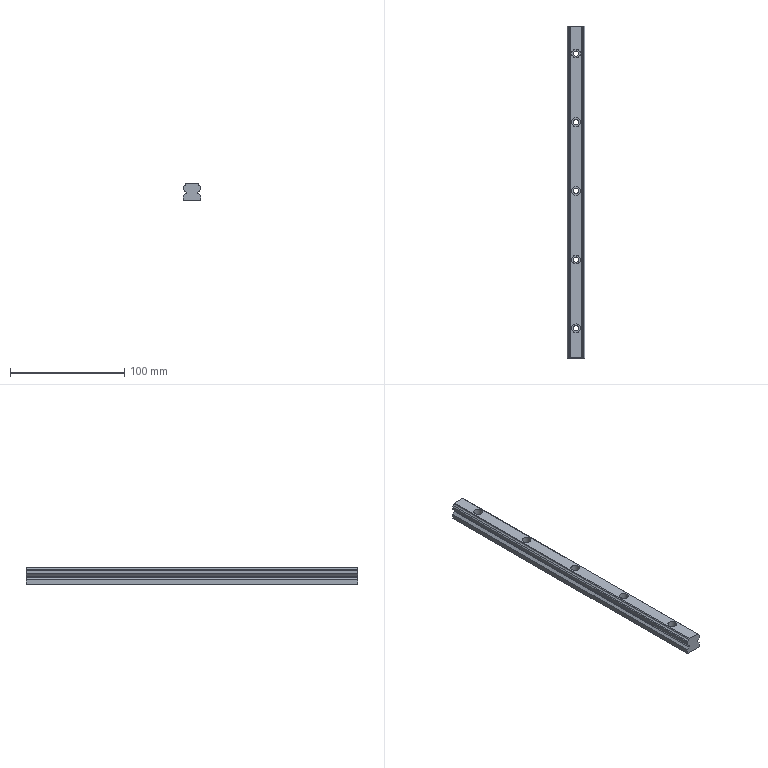Part | STEP file | Tube necking machine_id706_x_t | 1 solid | 37 faces | box 15 x 290 x 15 mm | volume 56751 mm3 | plane 19 | cylinder 18 | commonest cylinder face diameters 3 x6 4.5 x5 7.6 x5 1 x2